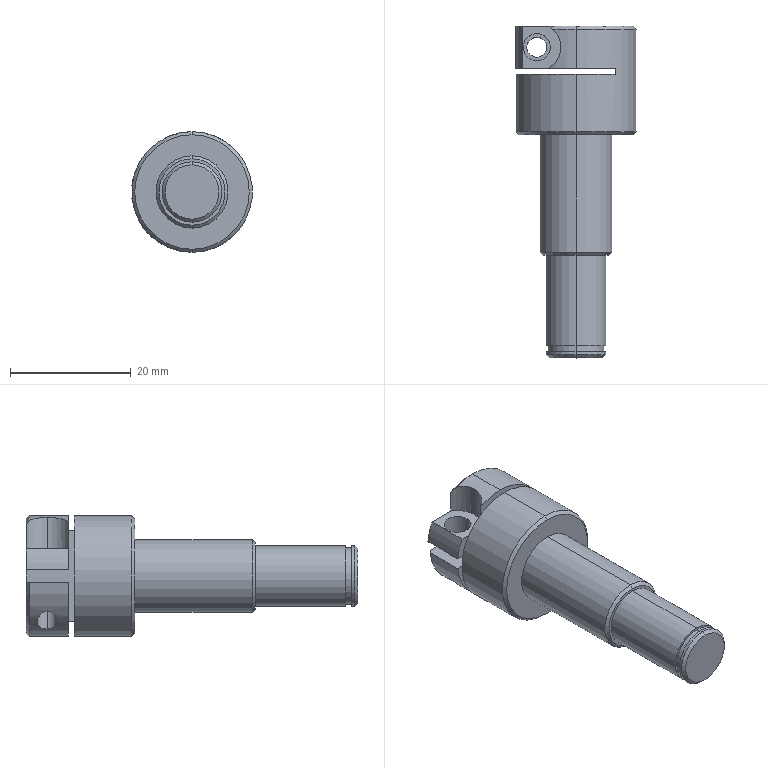Part | SolidWorks | features ICE 3, HoleWzd 2, Chamfer 1, Revolution 1 | 1 solid | 52 faces | box 20 x 55 x 20 mm | volume 7874 mm3 | cylinder 24 | plane 16 | cone 12 | commonest cylinder face diameters 8 x7 20 x5 10 x4 3.3 x2 4.5 x2 9.3 x2